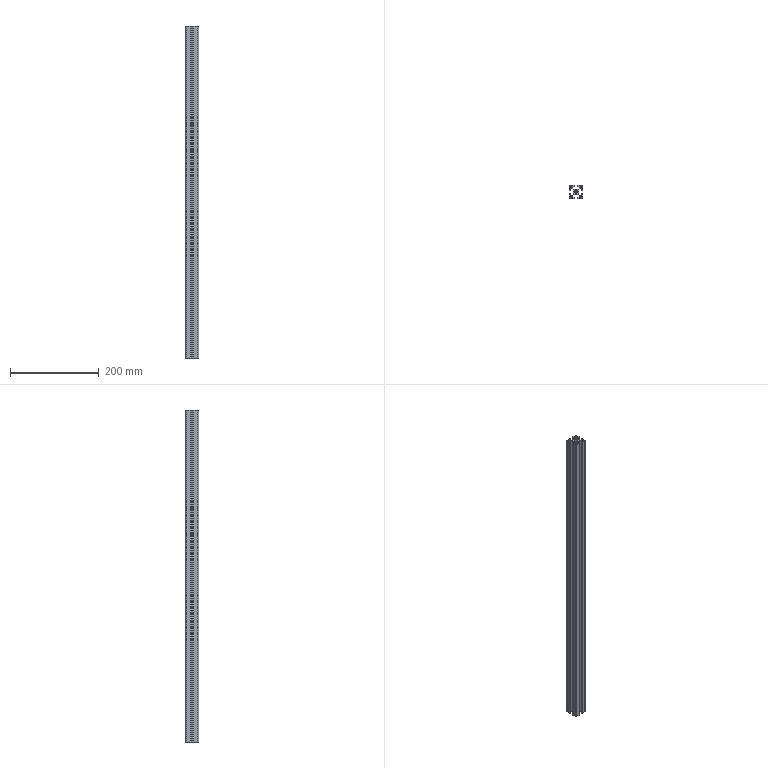Part | STEP file | ASND-0110-1-1 | 1 solid | 80 faces | box 30 x 30 x 749.1 mm | volume 248521 mm3 | plane 58 | cylinder 22 | commonest cylinder face diameters 0.6 x8 4.2 x8 4 x4 6.8 x2